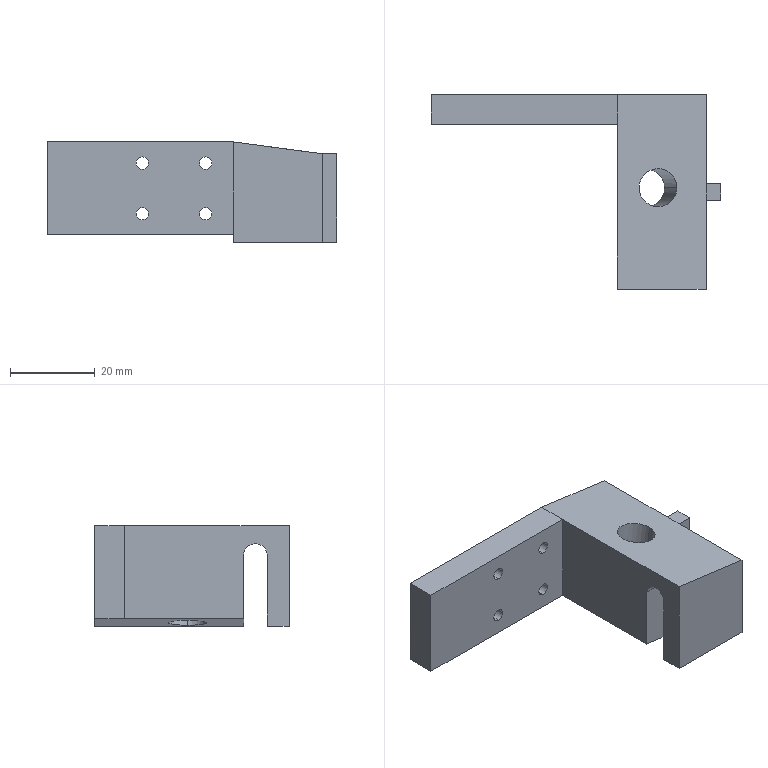Part | SolidWorks | features ICE 6, Extrusion 1 | 1 solid | 42 faces | box 68.51 x 46 x 23.69 mm | volume 24267 mm3 | plane 23 | cylinder 19 | commonest cylinder face diameters 2.9 x8 5 x8 9 x2 5.6 x1
STEP:
#1=CARTESIAN_POINT('',(-25.375,19.688,4.19));
#2=VERTEX_POINT('',#1);
#3=CARTESIAN_POINT('',(-25.375,19.688,9.19));
#4=VERTEX_POINT('',#3);
#5=CARTESIAN_POINT('',(-25.375,19.688,6.69));
#6=DIRECTION('',(0.,1.,0.));
#7=DIRECTION('',(0.,0.,1.));
#8=AXIS2_PLACEMENT_3D('',#5,#6,#7);
#9=CIRCLE('',#8,2.5);
#10=EDGE_CURVE('',#2,#4,#9,.T.);
#11=ORIENTED_EDGE('',*,*,#10,.F.);
#12=CARTESIAN_POINT('',(-25.375,22.688,4.19));
#13=VERTEX_POINT('',#12);
#14=CARTESIAN_POINT('',(-25.375,19.688,4.19));
#15=DIRECTION('',(0.,1.,0.));
#16=VECTOR('',#15,1000.);
#17=LINE('',#14,#16);
#18=EDGE_CURVE('',#2,#13,#17,.T.);
#19=ORIENTED_EDGE('',*,*,#18,.T.);
#20=CARTESIAN_POINT('',(-25.375,22.688,9.19));
#21=VERTEX_POINT('',#20);
#22=CARTESIAN_POINT('',(-25.375,22.688,6.69));
#23=DIRECTION('',(0.,1.,0.));
#24=DIRECTION('',(0.,0.,1.));
#25=AXIS2_PLACEMENT_3D('',#22,#23,#24);
#26=CIRCLE('',#25,2.5);
#27=EDGE_CURVE('',#13,#21,#26,.T.);
#28=ORIENTED_EDGE('',*,*,#27,.T.);
#29=CARTESIAN_POINT('',(-25.375,19.688,9.19));
#30=DIRECTION('',(0.,1.,0.));
#31=VECTOR('',#30,1000.);
#32=LINE('',#29,#31);
#33=EDGE_CURVE('',#4,#21,#32,.T.);
#34=ORIENTED_EDGE('',*,*,#33,.F.);
#35=EDGE_LOOP('',(#11,#19,#28,#34));
#36=FACE_OUTER_BOUND('',#35,.T.);
#37=CARTESIAN_POINT('',(-25.375,19.688,6.69));
#38=DIRECTION('',(0.,1.,0.));
#39=DIRECTION('',(0.,0.,1.));
#40=AXIS2_PLACEMENT_3D('',#37,#38,#39);
#41=CYLINDRICAL_SURFACE('',#40,2.5);
#42=ADVANCED_FACE('',(#36),#41,.F.);
#43=CARTESIAN_POINT('',(-10.375,19.688,16.19));
#44=VERTEX_POINT('',#43);
#45=CARTESIAN_POINT('',(-10.375,19.688,21.19));
#46=VERTEX_POINT('',#45);
#47=CARTESIAN_POINT('',(-10.375,19.688,18.69));
#48=DIRECTION('',(0.,1.,0.));
#49=DIRECTION('',(0.,0.,1.));
#50=AXIS2_PLACEMENT_3D('',#47,#48,#49);
#51=CIRCLE('',#50,2.5);
#52=EDGE_CURVE('',#44,#46,#51,.T.);
#53=ORIENTED_EDGE('',*,*,#52,.F.);
#54=CARTESIAN_POINT('',(-10.375,22.688,16.19));
#55=VERTEX_POINT('',#54);
#56=CARTESIAN_POINT('',(-10.375,19.688,16.19));
#57=DIRECTION('',(0.,1.,0.));
#58=VECTOR('',#57,1000.);
#59=LINE('',#56,#58);
#60=EDGE_CURVE('',#44,#55,#59,.T.);
#61=ORIENTED_EDGE('',*,*,#60,.T.);
#62=CARTESIAN_POINT('',(-10.375,22.688,21.19));
#63=VERTEX_POINT('',#62);
#64=CARTESIAN_POINT('',(-10.375,22.688,18.69));
#65=DIRECTION('',(0.,1.,0.));
#66=DIRECTION('',(0.,0.,1.));
#67=AXIS2_PLACEMENT_3D('',#64,#65,#66);
#68=CIRCLE('',#67,2.5);
#69=EDGE_CURVE('',#55,#63,#68,.T.);
#70=ORIENTED_EDGE('',*,*,#69,.T.);
#71=CARTESIAN_POINT('',(-10.375,19.688,21.19));
#72=DIRECTION('',(0.,1.,0.));
#73=VECTOR('',#72,1000.);
#74=LINE('',#71,#73);
#75=EDGE_CURVE('',#46,#63,#74,.T.);
#76=ORIENTED_EDGE('',*,*,#75,.F.);
#77=EDGE_LOOP('',(#53,#61,#70,#76));
#78=FACE_OUTER_BOUND('',#77,.T.);
#79=CARTESIAN_POINT('',(-10.375,19.688,18.69));
#80=DIRECTION('',(0.,1.,0.));
#81=DIRECTION('',(0.,0.,1.));
#82=AXIS2_PLACEMENT_3D('',#79,#80,#81);
#83=CYLINDRICAL_SURFACE('',#82,2.5);
#84=ADVANCED_FACE('',(#78),#83,.F.);
#85=CARTESIAN_POINT('',(-10.375,19.688,4.19));
#86=VERTEX_POINT('',#85);
#87=CARTESIAN_POINT('',(-10.375,19.688,9.19));
#88=VERTEX_POINT('',#87);
#89=CARTESIAN_POINT('',(-10.375,19.688,6.69));
#90=DIRECTION('',(0.,1.,0.));
#91=DIRECTION('',(0.,0.,1.));
#92=AXIS2_PLACEMENT_3D('',#89,#90,#91);
#93=CIRCLE('',#92,2.5);
#94=EDGE_CURVE('',#86,#88,#93,.T.);
#95=ORIENTED_EDGE('',*,*,#94,.F.);
#96=CARTESIAN_POINT('',(-10.375,22.688,4.19));
#97=VERTEX_POINT('',#96);
#98=CARTESIAN_POINT('',(-10.375,19.688,4.19));
#99=DIRECTION('',(0.,1.,0.));
#100=VECTOR('',#99,1000.);
#101=LINE('',#98,#100);
#102=EDGE_CURVE('',#86,#97,#101,.T.);
#103=ORIENTED_EDGE('',*,*,#102,.T.);
#104=CARTESIAN_POINT('',(-10.375,22.688,9.19));
#105=VERTEX_POINT('',#104);
#106=CARTESIAN_POINT('',(-10.375,22.688,6.69));
#107=DIRECTION('',(0.,1.,0.));
#108=DIRECTION('',(0.,0.,1.));
#109=AXIS2_PLACEMENT_3D('',#106,#107,#108);
#110=CIRCLE('',#109,2.5);
#111=EDGE_CURVE('',#97,#105,#110,.T.);
#112=ORIENTED_EDGE('',*,*,#111,.T.);
#113=CARTESIAN_POINT('',(-10.375,19.688,9.19));
#114=DIRECTION('',(0.,1.,0.));
#115=VECTOR('',#114,1000.);
#116=LINE('',#113,#115);
#117=EDGE_CURVE('',#88,#105,#116,.T.);
#118=ORIENTED_EDGE('',*,*,#117,.F.);
#119=EDGE_LOOP('',(#95,#103,#112,#118));
#120=FACE_OUTER_BOUND('',#119,.T.);
#121=CARTESIAN_POINT('',(-10.375,19.688,6.69));
#122=DIRECTION('',(0.,1.,0.));
#123=DIRECTION('',(0.,0.,1.));
#124=AXIS2_PLACEMENT_3D('',#121,#122,#123);
#125=CYLINDRICAL_SURFACE('',#124,2.5);
#126=ADVANCED_FACE('',(#120),#125,.F.);
#127=CARTESIAN_POINT('',(-25.375,19.688,16.19));
#128=VERTEX_POINT('',#127);
#129=CARTESIAN_POINT('',(-25.375,19.688,21.19));
#130=VERTEX_POINT('',#129);
#131=CARTESIAN_POINT('',(-25.375,19.688,18.69));
#132=DIRECTION('',(0.,1.,0.));
#133=DIRECTION('',(0.,0.,1.));
#134=AXIS2_PLACEMENT_3D('',#131,#132,#133);
#135=CIRCLE('',#134,2.5);
#136=EDGE_CURVE('',#128,#130,#135,.T.);
#137=ORIENTED_EDGE('',*,*,#136,.F.);
#138=CARTESIAN_POINT('',(-25.375,22.688,16.19));
#139=VERTEX_POINT('',#138);
#140=CARTESIAN_POINT('',(-25.375,19.688,16.19));
#141=DIRECTION('',(0.,1.,0.));
#142=VECTOR('',#141,1000.);
#143=LINE('',#140,#142);
#144=EDGE_CURVE('',#128,#139,#143,.T.);
#145=ORIENTED_EDGE('',*,*,#144,.T.);
#146=CARTESIAN_POINT('',(-25.375,22.688,21.19));
#147=VERTEX_POINT('',#146);
#148=CARTESIAN_POINT('',(-25.375,22.688,18.69));
#149=DIRECTION('',(0.,1.,0.));
#150=DIRECTION('',(0.,0.,1.));
#151=AXIS2_PLACEMENT_3D('',#148,#149,#150);
#152=CIRCLE('',#151,2.5);
#153=EDGE_CURVE('',#139,#147,#152,.T.);
#154=ORIENTED_EDGE('',*,*,#153,.T.);
#155=CARTESIAN_POINT('',(-25.375,19.688,21.19));
#156=DIRECTION('',(0.,1.,0.));
#157=VECTOR('',#156,1000.);
#158=LINE('',#155,#157);
#159=EDGE_CURVE('',#130,#147,#158,.T.);
#160=ORIENTED_EDGE('',*,*,#159,.F.);
#161=EDGE_LOOP('',(#137,#145,#154,#160));
#162=FACE_OUTER_BOUND('',#161,.T.);
#163=CARTESIAN_POINT('',(-25.375,19.688,18.69));
#164=DIRECTION('',(0.,1.,0.));
#165=DIRECTION('',(0.,0.,1.));
#166=AXIS2_PLACEMENT_3D('',#163,#164,#165);
#167=CYLINDRICAL_SURFACE('',#166,2.5);
#168=ADVANCED_FACE('',(#162),#167,.F.);
#169=CARTESIAN_POINT('',(1.295,0.6875,23.002));
#170=VERTEX_POINT('',#169);
#171=CARTESIAN_POINT('',(10.216,0.6875,21.813));
#172=VERTEX_POINT('',#171);
#173=CARTESIAN_POINT('',(1.295,0.6875,23.002));
#174=CARTESIAN_POINT('',(1.295,-8.313,23.002));
#175=CARTESIAN_POINT('',(10.216,-8.313,21.813));
#176=CARTESIAN_POINT('',(10.216,0.6875,21.813));
#177=(BOUNDED_CURVE()B_SPLINE_CURVE(3,(#173,#174,#175,#176),.UNSPECIFIED.,.F.,.T.)B_SPLINE_CURVE_WITH_KNOTS((4,4),(3.142,6.283),.UNSPECIFIED.)CURVE()GEOMETRIC_REPRESENTATION_ITEM()RATIONAL_B_SPLINE_CURVE((1.,0.3333,0.3333,1.))REPRESENTATION_ITEM(''));
#178=EDGE_CURVE('',#170,#172,#177,.T.);
#179=ORIENTED_EDGE('',*,*,#178,.T.);
#180=CARTESIAN_POINT('',(7.347,0.6875,0.2096));
#181=VERTEX_POINT('',#180);
#182=CARTESIAN_POINT('',(10.641,0.6875,25.018));
#183=DIRECTION('',(-0.1317,0.,-0.9913));
#184=VECTOR('',#183,1000.);
#185=LINE('',#182,#184);
#186=EDGE_CURVE('',#172,#181,#185,.T.);
#187=ORIENTED_EDGE('',*,*,#186,.T.);
#188=CARTESIAN_POINT('',(-1.575,0.6875,1.395));
#189=VERTEX_POINT('',#188);
#190=CARTESIAN_POINT('',(2.886,0.6875,0.8021));
#191=DIRECTION('',(-0.1317,0.,-0.9913));
#192=DIRECTION('',(-0.9913,0.,0.1317));
#193=AXIS2_PLACEMENT_3D('',#190,#191,#192);
#194=CIRCLE('',#193,4.5);
#195=EDGE_CURVE('',#181,#189,#194,.T.);
#196=ORIENTED_EDGE('',*,*,#195,.T.);
#197=CARTESIAN_POINT('',(1.72,0.6875,26.203));
#198=DIRECTION('',(-0.1317,0.,-0.9913));
#199=VECTOR('',#198,1000.);
#200=LINE('',#197,#199);
#201=EDGE_CURVE('',#170,#189,#200,.T.);
#202=ORIENTED_EDGE('',*,*,#201,.F.);
#203=EDGE_LOOP('',(#179,#187,#196,#202));
#204=FACE_OUTER_BOUND('',#203,.T.);
#205=CARTESIAN_POINT('',(6.181,0.6875,25.611));
#206=DIRECTION('',(-0.1317,0.,-0.9913));
#207=DIRECTION('',(-0.9913,0.,0.1317));
#208=AXIS2_PLACEMENT_3D('',#205,#206,#207);
#209=CYLINDRICAL_SURFACE('',#208,4.5);
#210=ADVANCED_FACE('',(#204),#209,.F.);
#211=CARTESIAN_POINT('',(-25.375,15.687,20.14));
#212=VERTEX_POINT('',#211);
#213=CARTESIAN_POINT('',(-25.375,15.687,17.24));
#214=VERTEX_POINT('',#213);
#215=CARTESIAN_POINT('',(-25.375,15.687,18.69));
#216=DIRECTION('',(0.,-1.,0.));
#217=DIRECTION('',(0.,0.,1.));
#218=AXIS2_PLACEMENT_3D('',#215,#216,#217);
#219=CIRCLE('',#218,1.45);
#220=EDGE_CURVE('',#212,#214,#219,.T.);
#221=ORIENTED_EDGE('',*,*,#220,.T.);
#222=CARTESIAN_POINT('',(-25.375,19.688,17.24));
#223=VERTEX_POINT('',#222);
#224=CARTESIAN_POINT('',(-25.375,-23.313,17.24));
#225=DIRECTION('',(0.,1.,0.));
#226=VECTOR('',#225,1000.);
#227=LINE('',#224,#226);
#228=EDGE_CURVE('',#214,#223,#227,.T.);
#229=ORIENTED_EDGE('',*,*,#228,.T.);
#230=CARTESIAN_POINT('',(-25.375,19.688,20.14));
#231=VERTEX_POINT('',#230);
#232=CARTESIAN_POINT('',(-25.375,19.688,18.69));
#233=DIRECTION('',(0.,-1.,0.));
#234=DIRECTION('',(0.,0.,1.));
#235=AXIS2_PLACEMENT_3D('',#232,#233,#234);
#236=CIRCLE('',#235,1.45);
#237=EDGE_CURVE('',#231,#223,#236,.T.);
#238=ORIENTED_EDGE('',*,*,#237,.F.);
#239=CARTESIAN_POINT('',(-25.375,-23.313,20.14));
#240=DIRECTION('',(0.,1.,0.));
#241=VECTOR('',#240,1000.);
#242=LINE('',#239,#241);
#243=EDGE_CURVE('',#212,#231,#242,.T.);
#244=ORIENTED_EDGE('',*,*,#243,.F.);
#245=EDGE_LOOP('',(#221,#229,#238,#244));
#246=FACE_OUTER_BOUND('',#245,.T.);
#247=CARTESIAN_POINT('',(-25.375,-23.313,18.69));
#248=DIRECTION('',(0.,1.,0.));
#249=DIRECTION('',(0.,0.,1.));
#250=AXIS2_PLACEMENT_3D('',#247,#248,#249);
#251=CYLINDRICAL_SURFACE('',#250,1.45);
#252=ADVANCED_FACE('',(#246),#251,.F.);
#253=CARTESIAN_POINT('',(-10.375,15.687,8.14));
#254=VERTEX_POINT('',#253);
#255=CARTESIAN_POINT('',(-10.375,15.687,5.24));
#256=VERTEX_POINT('',#255);
#257=CARTESIAN_POINT('',(-10.375,15.687,6.69));
#258=DIRECTION('',(0.,-1.,0.));
#259=DIRECTION('',(0.,0.,1.));
#260=AXIS2_PLACEMENT_3D('',#257,#258,#259);
#261=CIRCLE('',#260,1.45);
#262=EDGE_CURVE('',#254,#256,#261,.T.);
#263=ORIENTED_EDGE('',*,*,#262,.T.);
#264=CARTESIAN_POINT('',(-10.375,19.688,5.24));
#265=VERTEX_POINT('',#264);
#266=CARTESIAN_POINT('',(-10.375,-23.313,5.24));
#267=DIRECTION('',(0.,1.,0.));
#268=VECTOR('',#267,1000.);
#269=LINE('',#266,#268);
#270=EDGE_CURVE('',#256,#265,#269,.T.);
#271=ORIENTED_EDGE('',*,*,#270,.T.);
#272=CARTESIAN_POINT('',(-10.375,19.688,8.14));
#273=VERTEX_POINT('',#272);
#274=CARTESIAN_POINT('',(-10.375,19.688,6.69));
#275=DIRECTION('',(0.,-1.,0.));
#276=DIRECTION('',(0.,0.,1.));
#277=AXIS2_PLACEMENT_3D('',#274,#275,#276);
#278=CIRCLE('',#277,1.45);
#279=EDGE_CURVE('',#273,#265,#278,.T.);
#280=ORIENTED_EDGE('',*,*,#279,.F.);
#281=CARTESIAN_POINT('',(-10.375,-23.313,8.14));
#282=DIRECTION('',(0.,1.,0.));
#283=VECTOR('',#282,1000.);
#284=LINE('',#281,#283);
#285=EDGE_CURVE('',#254,#273,#284,.T.);
#286=ORIENTED_EDGE('',*,*,#285,.F.);
#287=EDGE_LOOP('',(#263,#271,#280,#286));
#288=FACE_OUTER_BOUND('',#287,.T.);
#289=CARTESIAN_POINT('',(-10.375,-23.313,6.69));
#290=DIRECTION('',(0.,1.,0.));
#291=DIRECTION('',(0.,0.,1.));
#292=AXIS2_PLACEMENT_3D('',#289,#290,#291);
#293=CYLINDRICAL_SURFACE('',#292,1.45);
#294=ADVANCED_FACE('',(#288),#293,.F.);
#295=CARTESIAN_POINT('',(-10.375,15.687,20.14));
#296=VERTEX_POINT('',#295);
#297=CARTESIAN_POINT('',(-10.375,15.687,17.24));
#298=VERTEX_POINT('',#297);
#299=CARTESIAN_POINT('',(-10.375,15.687,18.69));
#300=DIRECTION('',(0.,-1.,0.));
#301=DIRECTION('',(0.,0.,1.));
#302=AXIS2_PLACEMENT_3D('',#299,#300,#301);
#303=CIRCLE('',#302,1.45);
#304=EDGE_CURVE('',#296,#298,#303,.T.);
#305=ORIENTED_EDGE('',*,*,#304,.T.);
#306=CARTESIAN_POINT('',(-10.375,19.688,17.24));
#307=VERTEX_POINT('',#306);
#308=CARTESIAN_POINT('',(-10.375,-23.313,17.24));
#309=DIRECTION('',(0.,1.,0.));
#310=VECTOR('',#309,1000.);
#311=LINE('',#308,#310);
#312=EDGE_CURVE('',#298,#307,#311,.T.);
#313=ORIENTED_EDGE('',*,*,#312,.T.);
#314=CARTESIAN_POINT('',(-10.375,19.688,20.14));
#315=VERTEX_POINT('',#314);
#316=CARTESIAN_POINT('',(-10.375,19.688,18.69));
#317=DIRECTION('',(0.,-1.,0.));
#318=DIRECTION('',(0.,0.,1.));
#319=AXIS2_PLACEMENT_3D('',#316,#317,#318);
#320=CIRCLE('',#319,1.45);
#321=EDGE_CURVE('',#315,#307,#320,.T.);
#322=ORIENTED_EDGE('',*,*,#321,.F.);
#323=CARTESIAN_POINT('',(-10.375,-23.313,20.14));
#324=DIRECTION('',(0.,1.,0.));
#325=VECTOR('',#324,1000.);
#326=LINE('',#323,#325);
#327=EDGE_CURVE('',#296,#315,#326,.T.);
#328=ORIENTED_EDGE('',*,*,#327,.F.);
#329=EDGE_LOOP('',(#305,#313,#322,#328));
#330=FACE_OUTER_BOUND('',#329,.T.);
#331=CARTESIAN_POINT('',(-10.375,-23.313,18.69));
#332=DIRECTION('',(0.,1.,0.));
#333=DIRECTION('',(0.,0.,1.));
#334=AXIS2_PLACEMENT_3D('',#331,#332,#333);
#335=CYLINDRICAL_SURFACE('',#334,1.45);
#336=ADVANCED_FACE('',(#330),#335,.F.);
#337=CARTESIAN_POINT('',(-25.375,15.687,8.14));
#338=VERTEX_POINT('',#337);
#339=CARTESIAN_POINT('',(-25.375,15.687,5.24));
#340=VERTEX_POINT('',#339);
#341=CARTESIAN_POINT('',(-25.375,15.687,6.69));
#342=DIRECTION('',(0.,-1.,0.));
#343=DIRECTION('',(0.,0.,1.));
#344=AXIS2_PLACEMENT_3D('',#341,#342,#343);
#345=CIRCLE('',#344,1.45);
#346=EDGE_CURVE('',#338,#340,#345,.T.);
#347=ORIENTED_EDGE('',*,*,#346,.T.);
#348=CARTESIAN_POINT('',(-25.375,19.688,5.24));
#349=VERTEX_POINT('',#348);
#350=CARTESIAN_POINT('',(-25.375,-23.313,5.24));
#351=DIRECTION('',(0.,1.,0.));
#352=VECTOR('',#351,1000.);
#353=LINE('',#350,#352);
#354=EDGE_CURVE('',#340,#349,#353,.T.);
#355=ORIENTED_EDGE('',*,*,#354,.T.);
#356=CARTESIAN_POINT('',(-25.375,19.688,8.14));
#357=VERTEX_POINT('',#356);
#358=CARTESIAN_POINT('',(-25.375,19.688,6.69));
#359=DIRECTION('',(0.,-1.,0.));
#360=DIRECTION('',(0.,0.,1.));
#361=AXIS2_PLACEMENT_3D('',#358,#359,#360);
#362=CIRCLE('',#361,1.45);
#363=EDGE_CURVE('',#357,#349,#362,.T.);
#364=ORIENTED_EDGE('',*,*,#363,.F.);
#365=CARTESIAN_POINT('',(-25.375,-23.313,8.14));
#366=DIRECTION('',(0.,1.,0.));
#367=VECTOR('',#366,1000.);
#368=LINE('',#365,#367);
#369=EDGE_CURVE('',#338,#357,#368,.T.);
#370=ORIENTED_EDGE('',*,*,#369,.F.);
#371=EDGE_LOOP('',(#347,#355,#364,#370));
#372=FACE_OUTER_BOUND('',#371,.T.);
#373=CARTESIAN_POINT('',(-25.375,-23.313,6.69));
#374=DIRECTION('',(0.,1.,0.));
#375=DIRECTION('',(0.,0.,1.));
#376=AXIS2_PLACEMENT_3D('',#373,#374,#375);
#377=CYLINDRICAL_SURFACE('',#376,1.45);
#378=ADVANCED_FACE('',(#372),#377,.F.);
#379=ORIENTED_EDGE('',*,*,#354,.F.);
#380=CARTESIAN_POINT('',(-25.375,15.687,6.69));
#381=DIRECTION('',(0.,-1.,0.));
#382=DIRECTION('',(0.,0.,1.));
#383=AXIS2_PLACEMENT_3D('',#380,#381,#382);
#384=CIRCLE('',#383,1.45);
#385=EDGE_CURVE('',#340,#338,#384,.T.);
#386=ORIENTED_EDGE('',*,*,#385,.T.);
#387=ORIENTED_EDGE('',*,*,#369,.T.);
#388=CARTESIAN_POINT('',(-25.375,19.688,6.69));
#389=DIRECTION('',(0.,-1.,0.));
#390=DIRECTION('',(0.,0.,1.));
#391=AXIS2_PLACEMENT_3D('',#388,#389,#390);
#392=CIRCLE('',#391,1.45);
#393=EDGE_CURVE('',#349,#357,#392,.T.);
#394=ORIENTED_EDGE('',*,*,#393,.F.);
#395=EDGE_LOOP('',(#379,#386,#387,#394));
#396=FACE_OUTER_BOUND('',#395,.T.);
#397=CARTESIAN_POINT('',(-25.375,-23.313,6.69));
#398=DIRECTION('',(0.,1.,0.));
#399=DIRECTION('',(0.,0.,1.));
#400=AXIS2_PLACEMENT_3D('',#397,#398,#399);
#401=CYLINDRICAL_SURFACE('',#400,1.45);
#402=ADVANCED_FACE('',(#396),#401,.F.);
#403=ORIENTED_EDGE('',*,*,#312,.F.);
#404=CARTESIAN_POINT('',(-10.375,15.687,18.69));
#405=DIRECTION('',(0.,-1.,0.));
#406=DIRECTION('',(0.,0.,1.));
#407=AXIS2_PLACEMENT_3D('',#404,#405,#406);
#408=CIRCLE('',#407,1.45);
#409=EDGE_CURVE('',#298,#296,#408,.T.);
#410=ORIENTED_EDGE('',*,*,#409,.T.);
#411=ORIENTED_EDGE('',*,*,#327,.T.);
#412=CARTESIAN_POINT('',(-10.375,19.688,18.69));
#413=DIRECTION('',(0.,-1.,0.));
#414=DIRECTION('',(0.,0.,1.));
#415=AXIS2_PLACEMENT_3D('',#412,#413,#414);
#416=CIRCLE('',#415,1.45);
#417=EDGE_CURVE('',#307,#315,#416,.T.);
#418=ORIENTED_EDGE('',*,*,#417,.F.);
#419=EDGE_LOOP('',(#403,#410,#411,#418));
#420=FACE_OUTER_BOUND('',#419,.T.);
#421=CARTESIAN_POINT('',(-10.375,-23.313,18.69));
#422=DIRECTION('',(0.,1.,0.));
#423=DIRECTION('',(0.,0.,1.));
#424=AXIS2_PLACEMENT_3D('',#421,#422,#423);
#425=CYLINDRICAL_SURFACE('',#424,1.45);
#426=ADVANCED_FACE('',(#420),#425,.F.);
#427=ORIENTED_EDGE('',*,*,#270,.F.);
#428=CARTESIAN_POINT('',(-10.375,15.687,6.69));
#429=DIRECTION('',(0.,-1.,0.));
#430=DIRECTION('',(0.,0.,1.));
#431=AXIS2_PLACEMENT_3D('',#428,#429,#430);
#432=CIRCLE('',#431,1.45);
#433=EDGE_CURVE('',#256,#254,#432,.T.);
#434=ORIENTED_EDGE('',*,*,#433,.T.);
#435=ORIENTED_EDGE('',*,*,#285,.T.);
#436=CARTESIAN_POINT('',(-10.375,19.688,6.69));
#437=DIRECTION('',(0.,-1.,0.));
#438=DIRECTION('',(0.,0.,1.));
#439=AXIS2_PLACEMENT_3D('',#436,#437,#438);
#440=CIRCLE('',#439,1.45);
#441=EDGE_CURVE('',#265,#273,#440,.T.);
#442=ORIENTED_EDGE('',*,*,#441,.F.);
#443=EDGE_LOOP('',(#427,#434,#435,#442));
#444=FACE_OUTER_BOUND('',#443,.T.);
#445=CARTESIAN_POINT('',(-10.375,-23.313,6.69));
#446=DIRECTION('',(0.,1.,0.));
#447=DIRECTION('',(0.,0.,1.));
#448=AXIS2_PLACEMENT_3D('',#445,#446,#447);
#449=CYLINDRICAL_SURFACE('',#448,1.45);
#450=ADVANCED_FACE('',(#444),#449,.F.);
#451=ORIENTED_EDGE('',*,*,#228,.F.);
#452=CARTESIAN_POINT('',(-25.375,15.687,18.69));
#453=DIRECTION('',(0.,-1.,0.));
#454=DIRECTION('',(0.,0.,1.));
#455=AXIS2_PLACEMENT_3D('',#452,#453,#454);
#456=CIRCLE('',#455,1.45);
#457=EDGE_CURVE('',#214,#212,#456,.T.);
#458=ORIENTED_EDGE('',*,*,#457,.T.);
#459=ORIENTED_EDGE('',*,*,#243,.T.);
#460=CARTESIAN_POINT('',(-25.375,19.688,18.69));
#461=DIRECTION('',(0.,-1.,0.));
#462=DIRECTION('',(0.,0.,1.));
#463=AXIS2_PLACEMENT_3D('',#460,#461,#462);
#464=CIRCLE('',#463,1.45);
#465=EDGE_CURVE('',#223,#231,#464,.T.);
#466=ORIENTED_EDGE('',*,*,#465,.F.);
#467=EDGE_LOOP('',(#451,#458,#459,#466));
#468=FACE_OUTER_BOUND('',#467,.T.);
#469=CARTESIAN_POINT('',(-25.375,-23.313,18.69));
#470=DIRECTION('',(0.,1.,0.));
#471=DIRECTION('',(0.,0.,1.));
#472=AXIS2_PLACEMENT_3D('',#469,#470,#471);
#473=CYLINDRICAL_SURFACE('',#472,1.45);
#474=ADVANCED_FACE('',(#468),#473,.F.);
#475=CARTESIAN_POINT('',(-3.865,-23.312,0.));
#476=VERTEX_POINT('',#475);
#477=CARTESIAN_POINT('',(17.135,-23.312,0.));
#478=VERTEX_POINT('',#477);
#479=CARTESIAN_POINT('',(-47.875,-23.312,0.));
#480=DIRECTION('',(1.,0.,0.));
#481=VECTOR('',#480,1000.);
#482=LINE('',#479,#481);
#483=EDGE_CURVE('',#476,#478,#482,.T.);
#484=ORIENTED_EDGE('',*,*,#483,.F.);
#485=CARTESIAN_POINT('',(-3.865,-18.113,0.));
#486=VERTEX_POINT('',#485);
#487=CARTESIAN_POINT('',(-3.865,-23.312,0.));
#488=DIRECTION('',(0.,-1.,0.));
#489=VECTOR('',#488,1000.);
#490=LINE('',#487,#489);
#491=EDGE_CURVE('',#486,#476,#490,.T.);
#492=ORIENTED_EDGE('',*,*,#491,.F.);
#493=CARTESIAN_POINT('',(17.135,-18.113,0.));
#494=VERTEX_POINT('',#493);
#495=CARTESIAN_POINT('',(-47.876,-18.113,0.));
#496=DIRECTION('',(1.,0.,0.));
#497=VECTOR('',#496,1000.);
#498=LINE('',#495,#497);
#499=EDGE_CURVE('',#486,#494,#498,.T.);
#500=ORIENTED_EDGE('',*,*,#499,.T.);
#501=CARTESIAN_POINT('',(17.135,-2.312,0.));
#502=DIRECTION('',(0.,1.,0.));
#503=VECTOR('',#502,1000.);
#504=LINE('',#501,#503);
#505=EDGE_CURVE('',#478,#494,#504,.T.);
#506=ORIENTED_EDGE('',*,*,#505,.F.);
#507=EDGE_LOOP('',(#484,#492,#500,#506));
#508=FACE_OUTER_BOUND('',#507,.T.);
#509=CARTESIAN_POINT('',(0.,0.,0.));
#510=DIRECTION('',(0.,0.,1.));
#511=DIRECTION('',(1.,0.,0.));
#512=AXIS2_PLACEMENT_3D('',#509,#510,#511);
#513=PLANE('',#512);
#514=ADVANCED_FACE('',(#508),#513,.F.);
#515=CARTESIAN_POINT('',(-47.875,15.688,1.7));
#516=VERTEX_POINT('',#515);
#517=CARTESIAN_POINT('',(-47.875,22.688,1.7));
#518=VERTEX_POINT('',#517);
#519=CARTESIAN_POINT('',(-47.875,-23.313,1.7));
#520=DIRECTION('',(0.,1.,0.));
#521=VECTOR('',#520,1000.);
#522=LINE('',#519,#521);
#523=EDGE_CURVE('',#516,#518,#522,.T.);
#524=ORIENTED_EDGE('',*,*,#523,.F.);
#525=CARTESIAN_POINT('',(-47.875,15.688,23.69));
#526=VERTEX_POINT('',#525);
#527=CARTESIAN_POINT('',(-47.875,15.688,-0.001));
#528=DIRECTION('',(0.,0.,1.));
#529=VECTOR('',#528,1000.);
#530=LINE('',#527,#529);
#531=EDGE_CURVE('',#516,#526,#530,.T.);
#532=ORIENTED_EDGE('',*,*,#531,.T.);
#533=CARTESIAN_POINT('',(-47.875,22.688,23.69));
#534=VERTEX_POINT('',#533);
#535=CARTESIAN_POINT('',(-47.875,22.688,23.69));
#536=DIRECTION('',(0.,-1.,0.));
#537=VECTOR('',#536,1000.);
#538=LINE('',#535,#537);
#539=EDGE_CURVE('',#534,#526,#538,.T.);
#540=ORIENTED_EDGE('',*,*,#539,.F.);
#541=CARTESIAN_POINT('',(-47.875,22.688,23.69));
#542=DIRECTION('',(0.,0.,-1.));
#543=VECTOR('',#542,1000.);
#544=LINE('',#541,#543);
#545=EDGE_CURVE('',#534,#518,#544,.T.);
#546=ORIENTED_EDGE('',*,*,#545,.T.);
#547=EDGE_LOOP('',(#524,#532,#540,#546));
#548=FACE_OUTER_BOUND('',#547,.T.);
#549=CARTESIAN_POINT('',(-47.875,22.688,23.69));
#550=DIRECTION('',(1.,0.,0.));
#551=DIRECTION('',(0.,0.,-1.));
#552=AXIS2_PLACEMENT_3D('',#549,#550,#551);
#553=PLANE('',#552);
#554=ADVANCED_FACE('',(#548),#553,.F.);
#555=CARTESIAN_POINT('',(-3.865,-23.312,23.69));
#556=VERTEX_POINT('',#555);
#557=CARTESIAN_POINT('',(17.135,-23.312,20.89));
#558=VERTEX_POINT('',#557);
#559=CARTESIAN_POINT('',(17.135,-23.312,20.89));
#560=DIRECTION('',(0.9912,0.,-0.1322));
#561=VECTOR('',#560,1000.);
#562=LINE('',#559,#561);
#563=EDGE_CURVE('',#556,#558,#562,.T.);
#564=ORIENTED_EDGE('',*,*,#563,.F.);
#565=CARTESIAN_POINT('',(-3.865,-23.312,-0.001));
#566=DIRECTION('',(0.,0.,1.));
#567=VECTOR('',#566,1000.);
#568=LINE('',#565,#567);
#569=EDGE_CURVE('',#476,#556,#568,.T.);
#570=ORIENTED_EDGE('',*,*,#569,.F.);
#571=ORIENTED_EDGE('',*,*,#483,.T.);
#572=CARTESIAN_POINT('',(17.135,-23.312,-0.001));
#573=DIRECTION('',(0.,0.,1.));
#574=VECTOR('',#573,1000.);
#575=LINE('',#572,#574);
#576=EDGE_CURVE('',#478,#558,#575,.T.);
#577=ORIENTED_EDGE('',*,*,#576,.T.);
#578=EDGE_LOOP('',(#564,#570,#571,#577));
#579=FACE_OUTER_BOUND('',#578,.T.);
#580=CARTESIAN_POINT('',(-47.875,-23.312,23.69));
#581=DIRECTION('',(0.,1.,0.));
#582=DIRECTION('',(-1.,0.,0.));
#583=AXIS2_PLACEMENT_3D('',#580,#581,#582);
#584=PLANE('',#583);
#585=ADVANCED_FACE('',(#579),#584,.F.);
#586=CARTESIAN_POINT('',(20.635,-2.312,0.));
#587=VERTEX_POINT('',#586);
#588=CARTESIAN_POINT('',(20.635,1.688,0.));
#589=VERTEX_POINT('',#588);
#590=CARTESIAN_POINT('',(20.635,22.688,0.));
#591=DIRECTION('',(0.,1.,0.));
#592=VECTOR('',#591,1000.);
#593=LINE('',#590,#592);
#594=EDGE_CURVE('',#587,#589,#593,.T.);
#595=ORIENTED_EDGE('',*,*,#594,.T.);
#596=CARTESIAN_POINT('',(20.635,1.688,20.89));
#597=VERTEX_POINT('',#596);
#598=CARTESIAN_POINT('',(20.635,1.688,-0.001));
#599=DIRECTION('',(0.,0.,1.));
#600=VECTOR('',#599,1000.);
#601=LINE('',#598,#600);
#602=EDGE_CURVE('',#589,#597,#601,.T.);
#603=ORIENTED_EDGE('',*,*,#602,.T.);
#604=CARTESIAN_POINT('',(20.635,-2.312,20.89));
#605=VERTEX_POINT('',#604);
#606=CARTESIAN_POINT('',(20.635,-23.313,20.89));
#607=DIRECTION('',(0.,1.,0.));
#608=VECTOR('',#607,1000.);
#609=LINE('',#606,#608);
#610=EDGE_CURVE('',#605,#597,#609,.T.);
#611=ORIENTED_EDGE('',*,*,#610,.F.);
#612=CARTESIAN_POINT('',(20.635,-2.312,-0.001));
#613=DIRECTION('',(0.,0.,1.));
#614=VECTOR('',#613,1000.);
#615=LINE('',#612,#614);
#616=EDGE_CURVE('',#587,#605,#615,.T.);
#617=ORIENTED_EDGE('',*,*,#616,.F.);
#618=EDGE_LOOP('',(#595,#603,#611,#617));
#619=FACE_OUTER_BOUND('',#618,.T.);
#620=CARTESIAN_POINT('',(20.635,22.688,23.69));
#621=DIRECTION('',(-1.,0.,0.));
#622=DIRECTION('',(0.,0.,1.));
#623=AXIS2_PLACEMENT_3D('',#620,#621,#622);
#624=PLANE('',#623);
#625=ADVANCED_FACE('',(#619),#624,.F.);
#626=CARTESIAN_POINT('',(-10.375,22.688,6.69));
#627=DIRECTION('',(0.,1.,0.));
#628=DIRECTION('',(0.,0.,1.));
#629=AXIS2_PLACEMENT_3D('',#626,#627,#628);
#630=CIRCLE('',#629,2.5);
#631=EDGE_CURVE('',#105,#97,#630,.T.);
#632=ORIENTED_EDGE('',*,*,#631,.F.);
#633=ORIENTED_EDGE('',*,*,#111,.F.);
#634=EDGE_LOOP('',(#632,#633));
#635=FACE_BOUND('',#634,.T.);
#636=CARTESIAN_POINT('',(-25.375,22.688,18.69));
#637=DIRECTION('',(0.,1.,0.));
#638=DIRECTION('',(0.,0.,1.));
#639=AXIS2_PLACEMENT_3D('',#636,#637,#638);
#640=CIRCLE('',#639,2.5);
#641=EDGE_CURVE('',#147,#139,#640,.T.);
#642=ORIENTED_EDGE('',*,*,#641,.F.);
#643=ORIENTED_EDGE('',*,*,#153,.F.);
#644=EDGE_LOOP('',(#642,#643));
#645=FACE_BOUND('',#644,.T.);
#646=CARTESIAN_POINT('',(-10.375,22.688,18.69));
#647=DIRECTION('',(0.,1.,0.));
#648=DIRECTION('',(0.,0.,1.));
#649=AXIS2_PLACEMENT_3D('',#646,#647,#648);
#650=CIRCLE('',#649,2.5);
#651=EDGE_CURVE('',#63,#55,#650,.T.);
#652=ORIENTED_EDGE('',*,*,#651,.F.);
#653=ORIENTED_EDGE('',*,*,#69,.F.);
#654=EDGE_LOOP('',(#652,#653));
#655=FACE_BOUND('',#654,.T.);
#656=CARTESIAN_POINT('',(-25.375,22.688,6.69));
#657=DIRECTION('',(0.,1.,0.));
#658=DIRECTION('',(0.,0.,1.));
#659=AXIS2_PLACEMENT_3D('',#656,#657,#658);
#660=CIRCLE('',#659,2.5);
#661=EDGE_CURVE('',#21,#13,#660,.T.);
#662=ORIENTED_EDGE('',*,*,#661,.F.);
#663=ORIENTED_EDGE('',*,*,#27,.F.);
#664=EDGE_LOOP('',(#662,#663));
#665=FACE_BOUND('',#664,.T.);
#666=CARTESIAN_POINT('',(17.135,22.688,20.89));
#667=VERTEX_POINT('',#666);
#668=CARTESIAN_POINT('',(-3.865,22.688,23.69));
#669=VERTEX_POINT('',#668);
#670=CARTESIAN_POINT('',(17.135,22.688,20.89));
#671=DIRECTION('',(-0.9912,0.,0.1322));
#672=VECTOR('',#671,1000.);
#673=LINE('',#670,#672);
#674=EDGE_CURVE('',#667,#669,#673,.T.);
#675=ORIENTED_EDGE('',*,*,#674,.F.);
#676=CARTESIAN_POINT('',(17.135,22.688,0.));
#677=VERTEX_POINT('',#676);
#678=CARTESIAN_POINT('',(17.135,22.688,-0.001));
#679=DIRECTION('',(0.,0.,1.));
#680=VECTOR('',#679,1000.);
#681=LINE('',#678,#680);
#682=EDGE_CURVE('',#677,#667,#681,.T.);
#683=ORIENTED_EDGE('',*,*,#682,.F.);
#684=CARTESIAN_POINT('',(8.925,22.688,0.));
#685=VERTEX_POINT('',#684);
#686=CARTESIAN_POINT('',(-47.875,22.688,0.));
#687=DIRECTION('',(-1.,0.,0.));
#688=VECTOR('',#687,1000.);
#689=LINE('',#686,#688);
#690=EDGE_CURVE('',#677,#685,#689,.T.);
#691=ORIENTED_EDGE('',*,*,#690,.T.);
#692=CARTESIAN_POINT('',(-3.875,22.688,1.7));
#693=VERTEX_POINT('',#692);
#694=CARTESIAN_POINT('',(-3.875,22.688,1.7));
#695=DIRECTION('',(0.9913,0.,-0.1317));
#696=VECTOR('',#695,1000.);
#697=LINE('',#694,#696);
#698=EDGE_CURVE('',#693,#685,#697,.T.);
#699=ORIENTED_EDGE('',*,*,#698,.F.);
#700=CARTESIAN_POINT('',(-47.875,22.688,1.7));
#701=DIRECTION('',(1.,0.,0.));
#702=VECTOR('',#701,1000.);
#703=LINE('',#700,#702);
#704=EDGE_CURVE('',#518,#693,#703,.T.);
#705=ORIENTED_EDGE('',*,*,#704,.F.);
#706=ORIENTED_EDGE('',*,*,#545,.F.);
#707=CARTESIAN_POINT('',(-47.875,22.688,23.69));
#708=DIRECTION('',(-1.,0.,0.));
#709=VECTOR('',#708,1000.);
#710=LINE('',#707,#709);
#711=EDGE_CURVE('',#669,#534,#710,.T.);
#712=ORIENTED_EDGE('',*,*,#711,.F.);
#713=EDGE_LOOP('',(#675,#683,#691,#699,#705,#706,#712));
#714=FACE_OUTER_BOUND('',#713,.T.);
#715=CARTESIAN_POINT('',(-47.875,22.688,23.69));
#716=DIRECTION('',(0.,-1.,0.));
#717=DIRECTION('',(0.,0.,-1.));
#718=AXIS2_PLACEMENT_3D('',#715,#716,#717);
#719=PLANE('',#718);
#720=ADVANCED_FACE('',(#635,#645,#655,#665,#714),#719,.F.);
#721=CARTESIAN_POINT('',(-3.865,15.688,23.69));
#722=VERTEX_POINT('',#721);
#723=CARTESIAN_POINT('',(-3.865,15.688,23.69));
#724=DIRECTION('',(-1.,0.,0.));
#725=VECTOR('',#724,1000.);
#726=LINE('',#723,#725);
#727=EDGE_CURVE('',#722,#526,#726,.T.);
#728=ORIENTED_EDGE('',*,*,#727,.F.);
#729=CARTESIAN_POINT('',(-3.865,-23.313,23.69));
#730=DIRECTION('',(0.,1.,0.));
#731=VECTOR('',#730,1000.);
#732=LINE('',#729,#731);
#733=EDGE_CURVE('',#722,#669,#732,.T.);
#734=ORIENTED_EDGE('',*,*,#733,.T.);
#735=ORIENTED_EDGE('',*,*,#711,.T.);
#736=ORIENTED_EDGE('',*,*,#539,.T.);
#737=EDGE_LOOP('',(#728,#734,#735,#736));
#738=FACE_OUTER_BOUND('',#737,.T.);
#739=CARTESIAN_POINT('',(0.,0.,23.69));
#740=DIRECTION('',(0.,0.,1.));
#741=DIRECTION('',(1.,0.,0.));
#742=AXIS2_PLACEMENT_3D('',#739,#740,#741);
#743=PLANE('',#742);
#744=ADVANCED_FACE('',(#738),#743,.T.);
#745=CARTESIAN_POINT('',(17.135,1.688,0.));
#746=VERTEX_POINT('',#745);
#747=CARTESIAN_POINT('',(17.135,1.688,0.));
#748=DIRECTION('',(0.,1.,0.));
#749=VECTOR('',#748,1000.);
#750=LINE('',#747,#749);
#751=EDGE_CURVE('',#746,#677,#750,.T.);
#752=ORIENTED_EDGE('',*,*,#751,.F.);
#753=CARTESIAN_POINT('',(20.635,1.688,0.));
#754=DIRECTION('',(-1.,0.,0.));
#755=VECTOR('',#754,1000.);
#756=LINE('',#753,#755);
#757=EDGE_CURVE('',#589,#746,#756,.T.);
#758=ORIENTED_EDGE('',*,*,#757,.F.);
#759=ORIENTED_EDGE('',*,*,#594,.F.);
#760=CARTESIAN_POINT('',(17.135,-2.312,0.));
#761=VERTEX_POINT('',#760);
#762=CARTESIAN_POINT('',(20.635,-2.312,0.));
#763=DIRECTION('',(1.,0.,0.));
#764=VECTOR('',#763,1000.);
#765=LINE('',#762,#764);
#766=EDGE_CURVE('',#761,#587,#765,.T.);
#767=ORIENTED_EDGE('',*,*,#766,.F.);
#768=CARTESIAN_POINT('',(17.135,-12.513,0.));
#769=VERTEX_POINT('',#768);
#770=CARTESIAN_POINT('',(17.135,-2.312,0.));
#771=DIRECTION('',(0.,1.,0.));
#772=VECTOR('',#771,1000.);
#773=LINE('',#770,#772);
#774=EDGE_CURVE('',#769,#761,#773,.T.);
#775=ORIENTED_EDGE('',*,*,#774,.F.);
#776=CARTESIAN_POINT('',(8.925,-12.513,0.));
#777=VERTEX_POINT('',#776);
#778=CARTESIAN_POINT('',(-47.876,-12.513,0.));
#779=DIRECTION('',(1.,0.,0.));
#780=VECTOR('',#779,1000.);
#781=LINE('',#778,#780);
#782=EDGE_CURVE('',#777,#769,#781,.T.);
#783=ORIENTED_EDGE('',*,*,#782,.F.);
#784=CARTESIAN_POINT('',(8.925,-23.313,0.));
#785=DIRECTION('',(0.,1.,0.));
#786=VECTOR('',#785,1000.);
#787=LINE('',#784,#786);
#788=EDGE_CURVE('',#777,#685,#787,.T.);
#789=ORIENTED_EDGE('',*,*,#788,.T.);
#790=ORIENTED_EDGE('',*,*,#690,.F.);
#791=EDGE_LOOP('',(#752,#758,#759,#767,#775,#783,#789,#790));
#792=FACE_OUTER_BOUND('',#791,.T.);
#793=CARTESIAN_POINT('',(0.,0.,0.));
#794=DIRECTION('',(0.,0.,1.));
#795=DIRECTION('',(1.,0.,0.));
#796=AXIS2_PLACEMENT_3D('',#793,#794,#795);
#797=PLANE('',#796);
#798=ADVANCED_FACE('',(#792),#797,.F.);
#799=ORIENTED_EDGE('',*,*,#499,.F.);
#800=CARTESIAN_POINT('',(-3.865,-18.113,16.69));
#801=VERTEX_POINT('',#800);
#802=CARTESIAN_POINT('',(-3.865,-18.113,-0.001));
#803=DIRECTION('',(0.,0.,-1.));
#804=VECTOR('',#803,1000.);
#805=LINE('',#802,#804);
#806=EDGE_CURVE('',#801,#486,#805,.T.);
#807=ORIENTED_EDGE('',*,*,#806,.F.);
#808=CARTESIAN_POINT('',(17.135,-18.113,16.69));
#809=VERTEX_POINT('',#808);
#810=CARTESIAN_POINT('',(-47.876,-18.113,16.69));
#811=DIRECTION('',(1.,0.,0.));
#812=VECTOR('',#811,1000.);
#813=LINE('',#810,#812);
#814=EDGE_CURVE('',#801,#809,#813,.T.);
#815=ORIENTED_EDGE('',*,*,#814,.T.);
#816=CARTESIAN_POINT('',(17.135,-18.113,-0.001));
#817=DIRECTION('',(0.,0.,1.));
#818=VECTOR('',#817,1000.);
#819=LINE('',#816,#818);
#820=EDGE_CURVE('',#494,#809,#819,.T.);
#821=ORIENTED_EDGE('',*,*,#820,.F.);
#822=EDGE_LOOP('',(#799,#807,#815,#821));
#823=FACE_OUTER_BOUND('',#822,.T.);
#824=CARTESIAN_POINT('',(-47.876,-18.113,0.));
#825=DIRECTION('',(0.,-1.,0.));
#826=DIRECTION('',(0.,0.,-1.));
#827=AXIS2_PLACEMENT_3D('',#824,#825,#826);
#828=PLANE('',#827);
#829=ADVANCED_FACE('',(#823),#828,.F.);
#830=ORIENTED_EDGE('',*,*,#814,.F.);
#831=CARTESIAN_POINT('',(-3.865,-12.513,16.69));
#832=VERTEX_POINT('',#831);
#833=CARTESIAN_POINT('',(-3.865,-15.313,16.69));
#834=DIRECTION('',(1.,0.,0.));
#835=DIRECTION('',(0.,0.,-1.));
#836=AXIS2_PLACEMENT_3D('',#833,#834,#835);
#837=CIRCLE('',#836,2.8);
#838=EDGE_CURVE('',#832,#801,#837,.T.);
#839=ORIENTED_EDGE('',*,*,#838,.F.);
#840=CARTESIAN_POINT('',(17.135,-12.513,16.69));
#841=VERTEX_POINT('',#840);
#842=CARTESIAN_POINT('',(-47.876,-12.513,16.69));
#843=DIRECTION('',(1.,0.,0.));
#844=VECTOR('',#843,1000.);
#845=LINE('',#842,#844);
#846=EDGE_CURVE('',#832,#841,#845,.T.);
#847=ORIENTED_EDGE('',*,*,#846,.T.);
#848=CARTESIAN_POINT('',(17.135,-15.313,16.69));
#849=DIRECTION('',(-1.,0.,0.));
#850=DIRECTION('',(0.,0.,1.));
#851=AXIS2_PLACEMENT_3D('',#848,#849,#850);
#852=CIRCLE('',#851,2.8);
#853=EDGE_CURVE('',#809,#841,#852,.T.);
#854=ORIENTED_EDGE('',*,*,#853,.F.);
#855=EDGE_LOOP('',(#830,#839,#847,#854));
#856=FACE_OUTER_BOUND('',#855,.T.);
#857=CARTESIAN_POINT('',(-47.876,-15.313,16.69));
#858=DIRECTION('',(1.,0.,0.));
#859=DIRECTION('',(0.,1.,0.));
#860=AXIS2_PLACEMENT_3D('',#857,#858,#859);
#861=CYLINDRICAL_SURFACE('',#860,2.8);
#862=ADVANCED_FACE('',(#856),#861,.F.);
#863=ORIENTED_EDGE('',*,*,#846,.F.);
#864=CARTESIAN_POINT('',(-3.865,-12.513,1.699));
#865=VERTEX_POINT('',#864);
#866=CARTESIAN_POINT('',(-3.865,-12.513,-0.001));
#867=DIRECTION('',(0.,0.,1.));
#868=VECTOR('',#867,1000.);
#869=LINE('',#866,#868);
#870=EDGE_CURVE('',#865,#832,#869,.T.);
#871=ORIENTED_EDGE('',*,*,#870,.F.);
#872=CARTESIAN_POINT('',(-3.875,-12.513,1.7));
#873=DIRECTION('',(-0.9913,0.,0.1317));
#874=VECTOR('',#873,1000.);
#875=LINE('',#872,#874);
#876=EDGE_CURVE('',#777,#865,#875,.T.);
#877=ORIENTED_EDGE('',*,*,#876,.F.);
#878=ORIENTED_EDGE('',*,*,#782,.T.);
#879=CARTESIAN_POINT('',(17.135,-12.513,-0.001));
#880=DIRECTION('',(0.,0.,-1.));
#881=VECTOR('',#880,1000.);
#882=LINE('',#879,#881);
#883=EDGE_CURVE('',#841,#769,#882,.T.);
#884=ORIENTED_EDGE('',*,*,#883,.F.);
#885=EDGE_LOOP('',(#863,#871,#877,#878,#884));
#886=FACE_OUTER_BOUND('',#885,.T.);
#887=CARTESIAN_POINT('',(-47.876,-12.513,0.));
#888=DIRECTION('',(0.,1.,0.));
#889=DIRECTION('',(-1.,0.,0.));
#890=AXIS2_PLACEMENT_3D('',#887,#888,#889);
#891=PLANE('',#890);
#892=ADVANCED_FACE('',(#886),#891,.F.);
#893=CARTESIAN_POINT('',(-3.875,15.688,1.7));
#894=VERTEX_POINT('',#893);
#895=CARTESIAN_POINT('',(-3.875,-23.313,1.7));
#896=DIRECTION('',(0.,1.,0.));
#897=VECTOR('',#896,1000.);
#898=LINE('',#895,#897);
#899=EDGE_CURVE('',#894,#693,#898,.T.);
#900=ORIENTED_EDGE('',*,*,#899,.F.);
#901=CARTESIAN_POINT('',(-3.865,15.688,1.7));
#902=DIRECTION('',(1.,0.,0.));
#903=VECTOR('',#902,1000.);
#904=LINE('',#901,#903);
#905=EDGE_CURVE('',#516,#894,#904,.T.);
#906=ORIENTED_EDGE('',*,*,#905,.F.);
#907=ORIENTED_EDGE('',*,*,#523,.T.);
#908=ORIENTED_EDGE('',*,*,#704,.T.);
#909=EDGE_LOOP('',(#900,#906,#907,#908));
#910=FACE_OUTER_BOUND('',#909,.T.);
#911=CARTESIAN_POINT('',(-47.875,-23.313,1.7));
#912=DIRECTION('',(0.,0.,1.));
#913=DIRECTION('',(1.,0.,0.));
#914=AXIS2_PLACEMENT_3D('',#911,#912,#913);
#915=PLANE('',#914);
#916=ADVANCED_FACE('',(#910),#915,.F.);
#917=CARTESIAN_POINT('',(2.886,0.6875,0.8021));
#918=DIRECTION('',(-0.1317,0.,-0.9913));
#919=DIRECTION('',(-0.9913,0.,0.1317));
#920=AXIS2_PLACEMENT_3D('',#917,#918,#919);
#921=CIRCLE('',#920,4.5);
#922=EDGE_CURVE('',#189,#181,#921,.T.);
#923=ORIENTED_EDGE('',*,*,#922,.F.);
#924=ORIENTED_EDGE('',*,*,#195,.F.);
#925=EDGE_LOOP('',(#923,#924));
#926=FACE_BOUND('',#925,.T.);
#927=CARTESIAN_POINT('',(-3.865,15.688,1.699));
#928=VERTEX_POINT('',#927);
#929=CARTESIAN_POINT('',(-3.865,-23.312,1.699));
#930=DIRECTION('',(0.,-1.,0.));
#931=VECTOR('',#930,1000.);
#932=LINE('',#929,#931);
#933=EDGE_CURVE('',#928,#865,#932,.T.);
#934=ORIENTED_EDGE('',*,*,#933,.F.);
#935=CARTESIAN_POINT('',(-3.643,15.688,1.669));
#936=DIRECTION('',(0.9913,0.,-0.1317));
#937=VECTOR('',#936,1000.);
#938=LINE('',#935,#937);
#939=EDGE_CURVE('',#894,#928,#938,.T.);
#940=ORIENTED_EDGE('',*,*,#939,.F.);
#941=ORIENTED_EDGE('',*,*,#899,.T.);
#942=ORIENTED_EDGE('',*,*,#698,.T.);
#943=ORIENTED_EDGE('',*,*,#788,.F.);
#944=ORIENTED_EDGE('',*,*,#876,.T.);
#945=EDGE_LOOP('',(#934,#940,#941,#942,#943,#944));
#946=FACE_OUTER_BOUND('',#945,.T.);
#947=CARTESIAN_POINT('',(-3.875,-23.313,1.7));
#948=DIRECTION('',(0.1317,0.,0.9913));
#949=DIRECTION('',(0.9913,0.,-0.1317));
#950=AXIS2_PLACEMENT_3D('',#947,#948,#949);
#951=PLANE('',#950);
#952=ADVANCED_FACE('',(#926,#946),#951,.F.);
#953=ORIENTED_EDGE('',*,*,#178,.F.);
#954=CARTESIAN_POINT('',(10.216,0.6875,21.813));
#955=CARTESIAN_POINT('',(10.216,9.687,21.813));
#956=CARTESIAN_POINT('',(1.295,9.687,23.002));
#957=CARTESIAN_POINT('',(1.295,0.6875,23.002));
#958=(BOUNDED_CURVE()B_SPLINE_CURVE(3,(#954,#955,#956,#957),.UNSPECIFIED.,.F.,.T.)B_SPLINE_CURVE_WITH_KNOTS((4,4),(0.,3.142),.UNSPECIFIED.)CURVE()GEOMETRIC_REPRESENTATION_ITEM()RATIONAL_B_SPLINE_CURVE((1.,0.3333,0.3333,1.))REPRESENTATION_ITEM(''));
#959=EDGE_CURVE('',#172,#170,#958,.T.);
#960=ORIENTED_EDGE('',*,*,#959,.F.);
#961=EDGE_LOOP('',(#953,#960));
#962=FACE_BOUND('',#961,.T.);
#963=ORIENTED_EDGE('',*,*,#563,.T.);
#964=CARTESIAN_POINT('',(17.135,-2.312,20.89));
#965=VERTEX_POINT('',#964);
#966=CARTESIAN_POINT('',(17.135,-23.313,20.89));
#967=DIRECTION('',(0.,1.,0.));
#968=VECTOR('',#967,1000.);
#969=LINE('',#966,#968);
#970=EDGE_CURVE('',#558,#965,#969,.T.);
#971=ORIENTED_EDGE('',*,*,#970,.T.);
#972=CARTESIAN_POINT('',(17.135,1.688,20.89));
#973=VERTEX_POINT('',#972);
#974=CARTESIAN_POINT('',(17.135,-23.313,20.89));
#975=DIRECTION('',(0.,1.,0.));
#976=VECTOR('',#975,1000.);
#977=LINE('',#974,#976);
#978=EDGE_CURVE('',#965,#973,#977,.T.);
#979=ORIENTED_EDGE('',*,*,#978,.T.);
#980=CARTESIAN_POINT('',(17.135,-23.313,20.89));
#981=DIRECTION('',(0.,1.,0.));
#982=VECTOR('',#981,1000.);
#983=LINE('',#980,#982);
#984=EDGE_CURVE('',#973,#667,#983,.T.);
#985=ORIENTED_EDGE('',*,*,#984,.T.);
#986=ORIENTED_EDGE('',*,*,#674,.T.);
#987=ORIENTED_EDGE('',*,*,#733,.F.);
#988=CARTESIAN_POINT('',(-3.865,-23.313,23.69));
#989=DIRECTION('',(0.,1.,0.));
#990=VECTOR('',#989,1000.);
#991=LINE('',#988,#990);
#992=EDGE_CURVE('',#556,#722,#991,.T.);
#993=ORIENTED_EDGE('',*,*,#992,.F.);
#994=EDGE_LOOP('',(#963,#971,#979,#985,#986,#987,#993));
#995=FACE_OUTER_BOUND('',#994,.T.);
#996=CARTESIAN_POINT('',(17.135,-23.313,20.89));
#997=DIRECTION('',(-0.1322,0.,-0.9912));
#998=DIRECTION('',(-0.9912,0.,0.1322));
#999=AXIS2_PLACEMENT_3D('',#996,#997,#998);
#1000=PLANE('',#999);
#1001=ADVANCED_FACE('',(#962,#995),#1000,.F.);
#1002=ORIENTED_EDGE('',*,*,#610,.T.);
#1003=CARTESIAN_POINT('',(20.635,1.688,20.89));
#1004=DIRECTION('',(1.,0.,0.));
#1005=VECTOR('',#1004,1000.);
#1006=LINE('',#1003,#1005);
#1007=EDGE_CURVE('',#973,#597,#1006,.T.);
#1008=ORIENTED_EDGE('',*,*,#1007,.F.);
#1009=ORIENTED_EDGE('',*,*,#978,.F.);
#1010=CARTESIAN_POINT('',(20.635,-2.312,20.89));
#1011=DIRECTION('',(-1.,0.,0.));
#1012=VECTOR('',#1011,1000.);
#1013=LINE('',#1010,#1012);
#1014=EDGE_CURVE('',#605,#965,#1013,.T.);
#1015=ORIENTED_EDGE('',*,*,#1014,.F.);
#1016=EDGE_LOOP('',(#1002,#1008,#1009,#1015));
#1017=FACE_OUTER_BOUND('',#1016,.T.);
#1018=CARTESIAN_POINT('',(20.635,-23.313,20.89));
#1019=DIRECTION('',(0.,0.,-1.));
#1020=DIRECTION('',(-1.,0.,0.));
#1021=AXIS2_PLACEMENT_3D('',#1018,#1019,#1020);
#1022=PLANE('',#1021);
#1023=ADVANCED_FACE('',(#1017),#1022,.F.);
#1024=ORIENTED_EDGE('',*,*,#505,.T.);
#1025=ORIENTED_EDGE('',*,*,#820,.T.);
#1026=ORIENTED_EDGE('',*,*,#853,.T.);
#1027=ORIENTED_EDGE('',*,*,#883,.T.);
#1028=ORIENTED_EDGE('',*,*,#774,.T.);
#1029=CARTESIAN_POINT('',(17.135,-2.312,-0.001));
#1030=DIRECTION('',(0.,0.,1.));
#1031=VECTOR('',#1030,1000.);
#1032=LINE('',#1029,#1031);
#1033=EDGE_CURVE('',#761,#965,#1032,.T.);
#1034=ORIENTED_EDGE('',*,*,#1033,.T.);
#1035=ORIENTED_EDGE('',*,*,#970,.F.);
#1036=ORIENTED_EDGE('',*,*,#576,.F.);
#1037=EDGE_LOOP('',(#1024,#1025,#1026,#1027,#1028,#1034,#1035,#1036));
#1038=FACE_OUTER_BOUND('',#1037,.T.);
#1039=CARTESIAN_POINT('',(17.135,-2.312,-0.001));
#1040=DIRECTION('',(-1.,0.,0.));
#1041=DIRECTION('',(0.,0.,1.));
#1042=AXIS2_PLACEMENT_3D('',#1039,#1040,#1041);
#1043=PLANE('',#1042);
#1044=ADVANCED_FACE('',(#1038),#1043,.F.);
#1045=ORIENTED_EDGE('',*,*,#766,.T.);
#1046=ORIENTED_EDGE('',*,*,#616,.T.);
#1047=ORIENTED_EDGE('',*,*,#1014,.T.);
#1048=ORIENTED_EDGE('',*,*,#1033,.F.);
#1049=EDGE_LOOP('',(#1045,#1046,#1047,#1048));
#1050=FACE_OUTER_BOUND('',#1049,.T.);
#1051=CARTESIAN_POINT('',(20.635,-2.312,-0.001));
#1052=DIRECTION('',(0.,1.,0.));
#1053=DIRECTION('',(0.,0.,1.));
#1054=AXIS2_PLACEMENT_3D('',#1051,#1052,#1053);
#1055=PLANE('',#1054);
#1056=ADVANCED_FACE('',(#1050),#1055,.F.);
#1057=ORIENTED_EDGE('',*,*,#757,.T.);
#1058=CARTESIAN_POINT('',(17.135,1.688,-0.001));
#1059=DIRECTION('',(0.,0.,1.));
#1060=VECTOR('',#1059,1000.);
#1061=LINE('',#1058,#1060);
#1062=EDGE_CURVE('',#746,#973,#1061,.T.);
#1063=ORIENTED_EDGE('',*,*,#1062,.T.);
#1064=ORIENTED_EDGE('',*,*,#1007,.T.);
#1065=ORIENTED_EDGE('',*,*,#602,.F.);
#1066=EDGE_LOOP('',(#1057,#1063,#1064,#1065));
#1067=FACE_OUTER_BOUND('',#1066,.T.);
#1068=CARTESIAN_POINT('',(20.635,1.688,-0.001));
#1069=DIRECTION('',(0.,-1.,0.));
#1070=DIRECTION('',(0.,0.,-1.));
#1071=AXIS2_PLACEMENT_3D('',#1068,#1069,#1070);
#1072=PLANE('',#1071);
#1073=ADVANCED_FACE('',(#1067),#1072,.F.);
#1074=ORIENTED_EDGE('',*,*,#751,.T.);
#1075=ORIENTED_EDGE('',*,*,#682,.T.);
#1076=ORIENTED_EDGE('',*,*,#984,.F.);
#1077=ORIENTED_EDGE('',*,*,#1062,.F.);
#1078=EDGE_LOOP('',(#1074,#1075,#1076,#1077));
#1079=FACE_OUTER_BOUND('',#1078,.T.);
#1080=CARTESIAN_POINT('',(17.135,1.688,-0.001));
#1081=DIRECTION('',(-1.,0.,0.));
#1082=DIRECTION('',(0.,0.,1.));
#1083=AXIS2_PLACEMENT_3D('',#1080,#1081,#1082);
#1084=PLANE('',#1083);
#1085=ADVANCED_FACE('',(#1079),#1084,.F.);
#1086=ORIENTED_EDGE('',*,*,#220,.F.);
#1087=ORIENTED_EDGE('',*,*,#457,.F.);
#1088=EDGE_LOOP('',(#1086,#1087));
#1089=FACE_BOUND('',#1088,.T.);
#1090=ORIENTED_EDGE('',*,*,#262,.F.);
#1091=ORIENTED_EDGE('',*,*,#433,.F.);
#1092=EDGE_LOOP('',(#1090,#1091));
#1093=FACE_BOUND('',#1092,.T.);
#1094=ORIENTED_EDGE('',*,*,#304,.F.);
#1095=ORIENTED_EDGE('',*,*,#409,.F.);
#1096=EDGE_LOOP('',(#1094,#1095));
#1097=FACE_BOUND('',#1096,.T.);
#1098=ORIENTED_EDGE('',*,*,#346,.F.);
#1099=ORIENTED_EDGE('',*,*,#385,.F.);
#1100=EDGE_LOOP('',(#1098,#1099));
#1101=FACE_BOUND('',#1100,.T.);
#1102=ORIENTED_EDGE('',*,*,#905,.T.);
#1103=ORIENTED_EDGE('',*,*,#939,.T.);
#1104=CARTESIAN_POINT('',(-3.865,15.688,-0.001));
#1105=DIRECTION('',(0.,0.,1.));
#1106=VECTOR('',#1105,1000.);
#1107=LINE('',#1104,#1106);
#1108=EDGE_CURVE('',#928,#722,#1107,.T.);
#1109=ORIENTED_EDGE('',*,*,#1108,.T.);
#1110=ORIENTED_EDGE('',*,*,#727,.T.);
#1111=ORIENTED_EDGE('',*,*,#531,.F.);
#1112=EDGE_LOOP('',(#1102,#1103,#1109,#1110,#1111));
#1113=FACE_OUTER_BOUND('',#1112,.T.);
#1114=CARTESIAN_POINT('',(-3.865,15.688,-0.001));
#1115=DIRECTION('',(0.,1.,0.));
#1116=DIRECTION('',(0.,0.,1.));
#1117=AXIS2_PLACEMENT_3D('',#1114,#1115,#1116);
#1118=PLANE('',#1117);
#1119=ADVANCED_FACE('',(#1089,#1093,#1097,#1101,#1113),#1118,.F.);
#1120=ORIENTED_EDGE('',*,*,#491,.T.);
#1121=ORIENTED_EDGE('',*,*,#569,.T.);
#1122=ORIENTED_EDGE('',*,*,#992,.T.);
#1123=ORIENTED_EDGE('',*,*,#1108,.F.);
#1124=ORIENTED_EDGE('',*,*,#933,.T.);
#1125=ORIENTED_EDGE('',*,*,#870,.T.);
#1126=ORIENTED_EDGE('',*,*,#838,.T.);
#1127=ORIENTED_EDGE('',*,*,#806,.T.);
#1128=EDGE_LOOP('',(#1120,#1121,#1122,#1123,#1124,#1125,#1126,#1127));
#1129=FACE_OUTER_BOUND('',#1128,.T.);
#1130=CARTESIAN_POINT('',(-3.865,-23.312,-0.001));
#1131=DIRECTION('',(1.,0.,0.));
#1132=DIRECTION('',(0.,0.,-1.));
#1133=AXIS2_PLACEMENT_3D('',#1130,#1131,#1132);
#1134=PLANE('',#1133);
#1135=ADVANCED_FACE('',(#1129),#1134,.F.);
#1136=ORIENTED_EDGE('',*,*,#186,.F.);
#1137=ORIENTED_EDGE('',*,*,#959,.T.);
#1138=ORIENTED_EDGE('',*,*,#201,.T.);
#1139=ORIENTED_EDGE('',*,*,#922,.T.);
#1140=EDGE_LOOP('',(#1136,#1137,#1138,#1139));
#1141=FACE_OUTER_BOUND('',#1140,.T.);
#1142=CARTESIAN_POINT('',(6.181,0.6875,25.611));
#1143=DIRECTION('',(-0.1317,0.,-0.9913));
#1144=DIRECTION('',(-0.9913,0.,0.1317));
#1145=AXIS2_PLACEMENT_3D('',#1142,#1143,#1144);
#1146=CYLINDRICAL_SURFACE('',#1145,4.5);
#1147=ADVANCED_FACE('',(#1141),#1146,.F.);
#1148=CARTESIAN_POINT('',(-25.375,19.688,18.69));
#1149=DIRECTION('',(0.,1.,0.));
#1150=DIRECTION('',(0.,0.,1.));
#1151=AXIS2_PLACEMENT_3D('',#1148,#1149,#1150);
#1152=CIRCLE('',#1151,2.5);
#1153=EDGE_CURVE('',#130,#128,#1152,.T.);
#1154=ORIENTED_EDGE('',*,*,#1153,.T.);
#1155=ORIENTED_EDGE('',*,*,#136,.T.);
#1156=EDGE_LOOP('',(#1154,#1155));
#1157=FACE_OUTER_BOUND('',#1156,.T.);
#1158=ORIENTED_EDGE('',*,*,#237,.T.);
#1159=ORIENTED_EDGE('',*,*,#465,.T.);
#1160=EDGE_LOOP('',(#1158,#1159));
#1161=FACE_BOUND('',#1160,.T.);
#1162=CARTESIAN_POINT('',(-25.375,19.688,18.69));
#1163=DIRECTION('',(0.,1.,0.));
#1164=DIRECTION('',(0.,0.,1.));
#1165=AXIS2_PLACEMENT_3D('',#1162,#1163,#1164);
#1166=PLANE('',#1165);
#1167=ADVANCED_FACE('',(#1157,#1161),#1166,.T.);
#1168=ORIENTED_EDGE('',*,*,#144,.F.);
#1169=ORIENTED_EDGE('',*,*,#1153,.F.);
#1170=ORIENTED_EDGE('',*,*,#159,.T.);
#1171=ORIENTED_EDGE('',*,*,#641,.T.);
#1172=EDGE_LOOP('',(#1168,#1169,#1170,#1171));
#1173=FACE_OUTER_BOUND('',#1172,.T.);
#1174=CARTESIAN_POINT('',(-25.375,19.688,18.69));
#1175=DIRECTION('',(0.,1.,0.));
#1176=DIRECTION('',(0.,0.,1.));
#1177=AXIS2_PLACEMENT_3D('',#1174,#1175,#1176);
#1178=CYLINDRICAL_SURFACE('',#1177,2.5);
#1179=ADVANCED_FACE('',(#1173),#1178,.F.);
#1180=CARTESIAN_POINT('',(-10.375,19.688,6.69));
#1181=DIRECTION('',(0.,1.,0.));
#1182=DIRECTION('',(0.,0.,1.));
#1183=AXIS2_PLACEMENT_3D('',#1180,#1181,#1182);
#1184=CIRCLE('',#1183,2.5);
#1185=EDGE_CURVE('',#88,#86,#1184,.T.);
#1186=ORIENTED_EDGE('',*,*,#1185,.T.);
#1187=ORIENTED_EDGE('',*,*,#94,.T.);
#1188=EDGE_LOOP('',(#1186,#1187));
#1189=FACE_OUTER_BOUND('',#1188,.T.);
#1190=ORIENTED_EDGE('',*,*,#279,.T.);
#1191=ORIENTED_EDGE('',*,*,#441,.T.);
#1192=EDGE_LOOP('',(#1190,#1191));
#1193=FACE_BOUND('',#1192,.T.);
#1194=CARTESIAN_POINT('',(-10.375,19.688,6.69));
#1195=DIRECTION('',(0.,1.,0.));
#1196=DIRECTION('',(0.,0.,1.));
#1197=AXIS2_PLACEMENT_3D('',#1194,#1195,#1196);
#1198=PLANE('',#1197);
#1199=ADVANCED_FACE('',(#1189,#1193),#1198,.T.);
#1200=ORIENTED_EDGE('',*,*,#102,.F.);
#1201=ORIENTED_EDGE('',*,*,#1185,.F.);
#1202=ORIENTED_EDGE('',*,*,#117,.T.);
#1203=ORIENTED_EDGE('',*,*,#631,.T.);
#1204=EDGE_LOOP('',(#1200,#1201,#1202,#1203));
#1205=FACE_OUTER_BOUND('',#1204,.T.);
#1206=CARTESIAN_POINT('',(-10.375,19.688,6.69));
#1207=DIRECTION('',(0.,1.,0.));
#1208=DIRECTION('',(0.,0.,1.));
#1209=AXIS2_PLACEMENT_3D('',#1206,#1207,#1208);
#1210=CYLINDRICAL_SURFACE('',#1209,2.5);
#1211=ADVANCED_FACE('',(#1205),#1210,.F.);
#1212=CARTESIAN_POINT('',(-10.375,19.688,18.69));
#1213=DIRECTION('',(0.,1.,0.));
#1214=DIRECTION('',(0.,0.,1.));
#1215=AXIS2_PLACEMENT_3D('',#1212,#1213,#1214);
#1216=CIRCLE('',#1215,2.5);
#1217=EDGE_CURVE('',#46,#44,#1216,.T.);
#1218=ORIENTED_EDGE('',*,*,#1217,.T.);
#1219=ORIENTED_EDGE('',*,*,#52,.T.);
#1220=EDGE_LOOP('',(#1218,#1219));
#1221=FACE_OUTER_BOUND('',#1220,.T.);
#1222=ORIENTED_EDGE('',*,*,#321,.T.);
#1223=ORIENTED_EDGE('',*,*,#417,.T.);
#1224=EDGE_LOOP('',(#1222,#1223));
#1225=FACE_BOUND('',#1224,.T.);
#1226=CARTESIAN_POINT('',(-10.375,19.688,18.69));
#1227=DIRECTION('',(0.,1.,0.));
#1228=DIRECTION('',(0.,0.,1.));
#1229=AXIS2_PLACEMENT_3D('',#1226,#1227,#1228);
#1230=PLANE('',#1229);
#1231=ADVANCED_FACE('',(#1221,#1225),#1230,.T.);
#1232=ORIENTED_EDGE('',*,*,#60,.F.);
#1233=ORIENTED_EDGE('',*,*,#1217,.F.);
#1234=ORIENTED_EDGE('',*,*,#75,.T.);
#1235=ORIENTED_EDGE('',*,*,#651,.T.);
#1236=EDGE_LOOP('',(#1232,#1233,#1234,#1235));
#1237=FACE_OUTER_BOUND('',#1236,.T.);
#1238=CARTESIAN_POINT('',(-10.375,19.688,18.69));
#1239=DIRECTION('',(0.,1.,0.));
#1240=DIRECTION('',(0.,0.,1.));
#1241=AXIS2_PLACEMENT_3D('',#1238,#1239,#1240);
#1242=CYLINDRICAL_SURFACE('',#1241,2.5);
#1243=ADVANCED_FACE('',(#1237),#1242,.F.);
#1244=CARTESIAN_POINT('',(-25.375,19.688,6.69));
#1245=DIRECTION('',(0.,1.,0.));
#1246=DIRECTION('',(0.,0.,1.));
#1247=AXIS2_PLACEMENT_3D('',#1244,#1245,#1246);
#1248=CIRCLE('',#1247,2.5);
#1249=EDGE_CURVE('',#4,#2,#1248,.T.);
#1250=ORIENTED_EDGE('',*,*,#1249,.T.);
#1251=ORIENTED_EDGE('',*,*,#10,.T.);
#1252=EDGE_LOOP('',(#1250,#1251));
#1253=FACE_OUTER_BOUND('',#1252,.T.);
#1254=ORIENTED_EDGE('',*,*,#363,.T.);
#1255=ORIENTED_EDGE('',*,*,#393,.T.);
#1256=EDGE_LOOP('',(#1254,#1255));
#1257=FACE_BOUND('',#1256,.T.);
#1258=CARTESIAN_POINT('',(-25.375,19.688,6.69));
#1259=DIRECTION('',(0.,1.,0.));
#1260=DIRECTION('',(0.,0.,1.));
#1261=AXIS2_PLACEMENT_3D('',#1258,#1259,#1260);
#1262=PLANE('',#1261);
#1263=ADVANCED_FACE('',(#1253,#1257),#1262,.T.);
#1264=ORIENTED_EDGE('',*,*,#18,.F.);
#1265=ORIENTED_EDGE('',*,*,#1249,.F.);
#1266=ORIENTED_EDGE('',*,*,#33,.T.);
#1267=ORIENTED_EDGE('',*,*,#661,.T.);
#1268=EDGE_LOOP('',(#1264,#1265,#1266,#1267));
#1269=FACE_OUTER_BOUND('',#1268,.T.);
#1270=CARTESIAN_POINT('',(-25.375,19.688,6.69));
#1271=DIRECTION('',(0.,1.,0.));
#1272=DIRECTION('',(0.,0.,1.));
#1273=AXIS2_PLACEMENT_3D('',#1270,#1271,#1272);
#1274=CYLINDRICAL_SURFACE('',#1273,2.5);
#1275=ADVANCED_FACE('',(#1269),#1274,.F.);
#1276=CLOSED_SHELL('',(#42,#84,#126,#168,#210,#252,#294,#336,#378,#402,#426,#450,#474,#514,#554,#585,#625,#720,#744,#798,#829,#862,#892,#916,#952,#1001,#1023,#1044,#1056,#1073,#1085,#1119,#1135,#1147,#1167,#1179,#1199,#1211,#1231,#1243,#1263,#1275));
#1277=MANIFOLD_SOLID_BREP('',#1276);
#1278=CARTESIAN_POINT('',(0.,0.,0.));
#1279=DIRECTION('',(0.,0.,1.));
#1280=DIRECTION('',(1.,0.,0.));
#1281=AXIS2_PLACEMENT_3D('',#1278,#1279,#1280);
#1282=(LENGTH_UNIT()NAMED_UNIT(*)SI_UNIT(.MILLI.,.METRE.));
#1283=UNCERTAINTY_MEASURE_WITH_UNIT(LENGTH_MEASURE(0.00001),#1282,'','');
#1284=(NAMED_UNIT(*)PLANE_ANGLE_UNIT()SI_UNIT($,.RADIAN.));
#1285=(NAMED_UNIT(*)SI_UNIT($,.STERADIAN.)SOLID_ANGLE_UNIT());
#1286=(GEOMETRIC_REPRESENTATION_CONTEXT(3)GLOBAL_UNCERTAINTY_ASSIGNED_CONTEXT((#1283))GLOBAL_UNIT_ASSIGNED_CONTEXT((#1282,#1284,#1285))REPRESENTATION_CONTEXT('',''));
#1287=ADVANCED_BREP_SHAPE_REPRESENTATION('',(#1277,#1281),#1286);